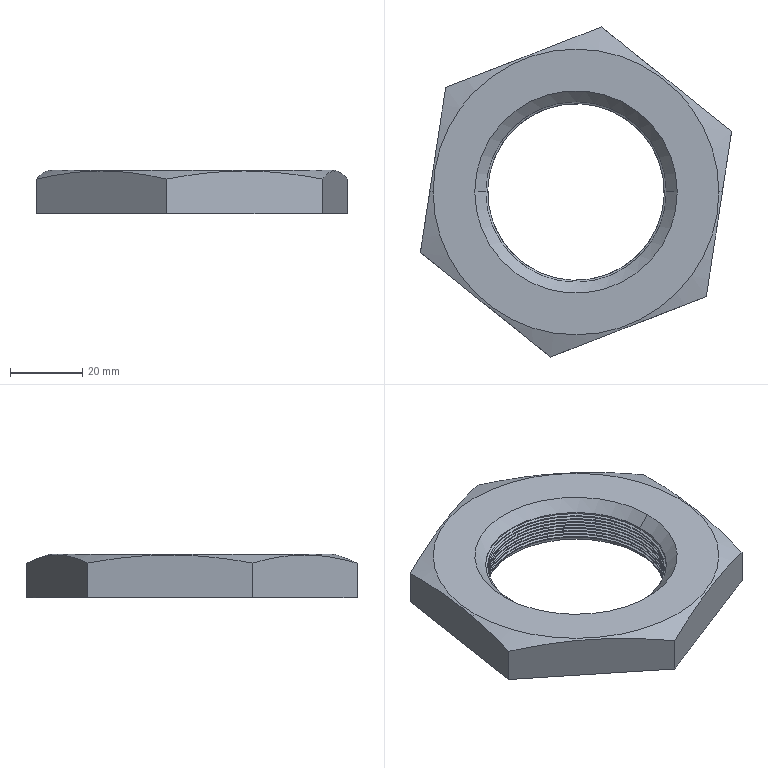Part | STEP file | Adjusting nut 1 | 1 solid | 35 faces | box 86.085 x 91.305 x 12 mm | volume 42133 mm3 | cylinder 18 | plane 10 | cone 4 | spline 3 | commonest cylinder face diameters 50 x18